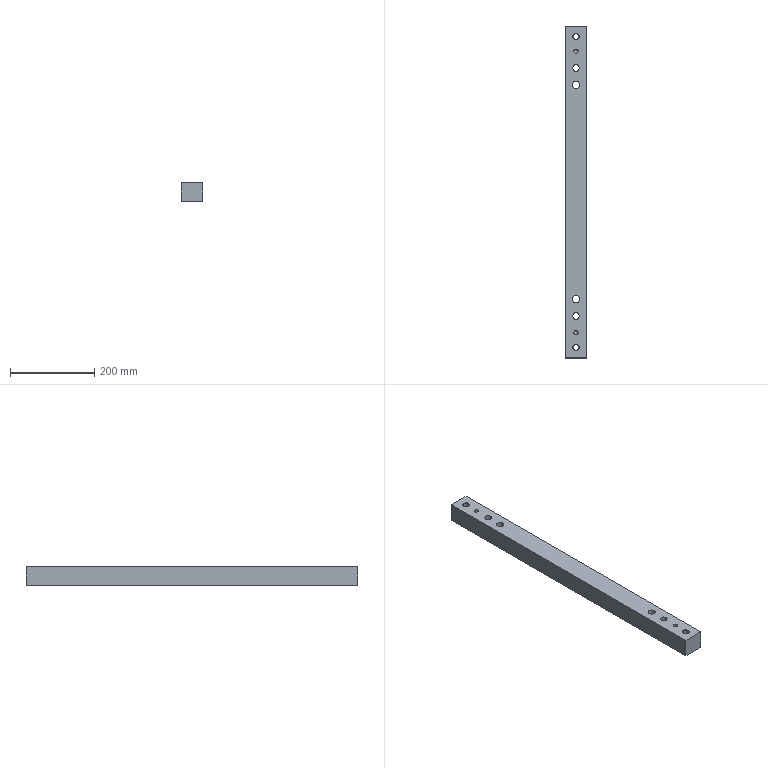Part | STEP file | 026_id2218_x_t | 1 solid | 18 faces | box 50 x 790 x 45 mm | volume 1720407 mm3 | cylinder 8 | plane 6 | cone 4 | commonest cylinder face diameters 10.3 x2 14 x2 16 x2 17 x2
STEP:
#1=CARTESIAN_POINT('',(0.,0.,0.));
#2=DIRECTION('',(0.,0.,1.));
#3=DIRECTION('',(1.,0.,0.));
#4=AXIS2_PLACEMENT_3D('',#1,#2,#3);
#5=CARTESIAN_POINT('',(1285.,-255.,185.));
#6=VERTEX_POINT('',#5);
#7=CARTESIAN_POINT('',(1293.5,-255.,185.));
#8=DIRECTION('',(0.,0.,1.));
#9=DIRECTION('',(-1.,0.,0.));
#10=AXIS2_PLACEMENT_3D('',#7,#8,#9);
#11=CIRCLE('',#10,8.5);
#12=CARTESIAN_POINT('',(193.5,0.,185.));
#13=DIRECTION('',(0.,0.,-1.));
#14=DIRECTION('',(1.,0.,0.));
#15=AXIS2_PLACEMENT_3D('',#12,#13,#14);
#16=PLANE('',#15);
#17=CARTESIAN_POINT('',(1091.5,255.));
#18=CARTESIAN_POINT('',(1091.5,269.722));
#19=CARTESIAN_POINT('',(1104.25,262.361));
#20=CARTESIAN_POINT('',(1117.,255.));
#21=CARTESIAN_POINT('',(1104.25,247.639));
#22=CARTESIAN_POINT('',(1091.5,240.278));
#23=CARTESIAN_POINT('',(1091.5,255.));
#24=(BOUNDED_CURVE()B_SPLINE_CURVE(2,(#17,#18,#19,#20,#21,#22,#23),.UNSPECIFIED.,.T.,.F.)B_SPLINE_CURVE_WITH_KNOTS((1,2,2,2,2,1),(-2.094,0.,2.094,4.189,6.283,8.378),.UNSPECIFIED.)CURVE()GEOMETRIC_REPRESENTATION_ITEM()RATIONAL_B_SPLINE_CURVE((1.,0.5,1.,0.5,1.,0.5,1.))REPRESENTATION_ITEM(''));
#25=(GEOMETRIC_REPRESENTATION_CONTEXT(2)PARAMETRIC_REPRESENTATION_CONTEXT()REPRESENTATION_CONTEXT('',''));
#26=DEFINITIONAL_REPRESENTATION('',(#24),#25);
#27=PCURVE('',#16,#26);
#28=CARTESIAN_POINT('',(1293.5,-255.,150.));
#29=DIRECTION('',(0.,0.,1.));
#30=DIRECTION('',(1.,0.,0.));
#31=AXIS2_PLACEMENT_3D('',#28,#29,#30);
#32=CYLINDRICAL_SURFACE('',#31,8.5);
#33=CARTESIAN_POINT('',(3.142,35.));
#34=DIRECTION('',(1.,0.));
#35=VECTOR('',#34,1.);
#36=LINE('',#33,#35);
#37=(GEOMETRIC_REPRESENTATION_CONTEXT(2)PARAMETRIC_REPRESENTATION_CONTEXT()REPRESENTATION_CONTEXT('',''));
#38=DEFINITIONAL_REPRESENTATION('',(#36),#37);
#39=PCURVE('',#32,#38);
#40=SURFACE_CURVE('',#11,(#27,#39),.PCURVE_S1.);
#41=EDGE_CURVE('',#6,#6,#40,.T.);
#42=ORIENTED_EDGE('',*,*,#41,.T.);
#43=EDGE_LOOP('',(#42));
#44=FACE_BOUND('',#43,.T.);
#45=CARTESIAN_POINT('',(1286.5,-370.,185.));
#46=VERTEX_POINT('',#45);
#47=CARTESIAN_POINT('',(1293.5,-370.,185.));
#48=DIRECTION('',(0.,0.,-1.));
#49=DIRECTION('',(-1.,0.,0.));
#50=AXIS2_PLACEMENT_3D('',#47,#48,#49);
#51=CIRCLE('',#50,7.);
#52=CARTESIAN_POINT('',(1100.,370.));
#53=DIRECTION('',(-1.,0.));
#54=AXIS2_PLACEMENT_2D('',#52,#53);
#55=CIRCLE('',#54,7.);
#56=(GEOMETRIC_REPRESENTATION_CONTEXT(2)PARAMETRIC_REPRESENTATION_CONTEXT()REPRESENTATION_CONTEXT('',''));
#57=DEFINITIONAL_REPRESENTATION('',(#55),#56);
#58=PCURVE('',#16,#57);
#59=CARTESIAN_POINT('',(1293.5,-370.,230.));
#60=DIRECTION('',(0.,0.,-1.));
#61=DIRECTION('',(-1.,0.,0.));
#62=AXIS2_PLACEMENT_3D('',#59,#60,#61);
#63=CYLINDRICAL_SURFACE('',#62,7.);
#64=CARTESIAN_POINT('',(0.,45.));
#65=DIRECTION('',(1.,0.));
#66=VECTOR('',#65,1.);
#67=LINE('',#64,#66);
#68=(GEOMETRIC_REPRESENTATION_CONTEXT(2)PARAMETRIC_REPRESENTATION_CONTEXT()REPRESENTATION_CONTEXT('',''));
#69=DEFINITIONAL_REPRESENTATION('',(#67),#68);
#70=PCURVE('',#63,#69);
#71=SURFACE_CURVE('',#51,(#58,#70),.PCURVE_S1.);
#72=EDGE_CURVE('',#46,#46,#71,.T.);
#73=ORIENTED_EDGE('',*,*,#72,.F.);
#74=EDGE_LOOP('',(#73));
#75=FACE_BOUND('',#74,.T.);
#76=CARTESIAN_POINT('',(1318.5,395.,185.));
#77=VERTEX_POINT('',#76);
#78=CARTESIAN_POINT('',(1318.5,-395.,185.));
#79=VERTEX_POINT('',#78);
#80=CARTESIAN_POINT('',(1318.5,0.,185.));
#81=DIRECTION('',(0.,-1.,0.));
#82=VECTOR('',#81,1.);
#83=LINE('',#80,#82);
#84=CARTESIAN_POINT('',(1125.,0.));
#85=DIRECTION('',(0.,1.));
#86=VECTOR('',#85,1.);
#87=LINE('',#84,#86);
#88=(GEOMETRIC_REPRESENTATION_CONTEXT(2)PARAMETRIC_REPRESENTATION_CONTEXT()REPRESENTATION_CONTEXT('',''));
#89=DEFINITIONAL_REPRESENTATION('',(#87),#88);
#90=PCURVE('',#16,#89);
#91=CARTESIAN_POINT('',(1318.5,-210.,-28.5));
#92=DIRECTION('',(1.,0.,0.));
#93=DIRECTION('',(0.,0.,1.));
#94=AXIS2_PLACEMENT_3D('',#91,#92,#93);
#95=PLANE('',#94);
#96=CARTESIAN_POINT('',(213.5,-210.));
#97=DIRECTION('',(0.,1.));
#98=VECTOR('',#97,1.);
#99=LINE('',#96,#98);
#100=(GEOMETRIC_REPRESENTATION_CONTEXT(2)PARAMETRIC_REPRESENTATION_CONTEXT()REPRESENTATION_CONTEXT('',''));
#101=DEFINITIONAL_REPRESENTATION('',(#99),#100);
#102=PCURVE('',#95,#101);
#103=SURFACE_CURVE('',#83,(#90,#102),.PCURVE_S1.);
#104=EDGE_CURVE('',#77,#79,#103,.T.);
#105=ORIENTED_EDGE('',*,*,#104,.T.);
#106=CARTESIAN_POINT('',(1268.5,-395.,185.));
#107=VERTEX_POINT('',#106);
#108=CARTESIAN_POINT('',(193.5,-395.,185.));
#109=DIRECTION('',(1.,0.,0.));
#110=VECTOR('',#109,1.);
#111=LINE('',#108,#110);
#112=CARTESIAN_POINT('',(0.,395.));
#113=DIRECTION('',(1.,0.));
#114=VECTOR('',#113,1.);
#115=LINE('',#112,#114);
#116=(GEOMETRIC_REPRESENTATION_CONTEXT(2)PARAMETRIC_REPRESENTATION_CONTEXT()REPRESENTATION_CONTEXT('',''));
#117=DEFINITIONAL_REPRESENTATION('',(#115),#116);
#118=PCURVE('',#16,#117);
#119=CARTESIAN_POINT('',(1318.5,-395.,-28.5));
#120=DIRECTION('',(0.,1.,0.));
#121=DIRECTION('',(0.,0.,-1.));
#122=AXIS2_PLACEMENT_3D('',#119,#120,#121);
#123=PLANE('',#122);
#124=CARTESIAN_POINT('',(-213.5,1125.));
#125=DIRECTION('',(0.,-1.));
#126=VECTOR('',#125,1.);
#127=LINE('',#124,#126);
#128=(GEOMETRIC_REPRESENTATION_CONTEXT(2)PARAMETRIC_REPRESENTATION_CONTEXT()REPRESENTATION_CONTEXT('',''));
#129=DEFINITIONAL_REPRESENTATION('',(#127),#128);
#130=PCURVE('',#123,#129);
#131=SURFACE_CURVE('',#111,(#118,#130),.PCURVE_S1.);
#132=EDGE_CURVE('',#107,#79,#131,.T.);
#133=ORIENTED_EDGE('',*,*,#132,.F.);
#134=CARTESIAN_POINT('',(1268.5,395.,185.));
#135=VERTEX_POINT('',#134);
#136=CARTESIAN_POINT('',(1268.5,-210.,185.));
#137=DIRECTION('',(0.,1.,0.));
#138=VECTOR('',#137,1.);
#139=LINE('',#136,#138);
#140=CARTESIAN_POINT('',(1075.,210.));
#141=DIRECTION('',(0.,-1.));
#142=VECTOR('',#141,1.);
#143=LINE('',#140,#142);
#144=(GEOMETRIC_REPRESENTATION_CONTEXT(2)PARAMETRIC_REPRESENTATION_CONTEXT()REPRESENTATION_CONTEXT('',''));
#145=DEFINITIONAL_REPRESENTATION('',(#143),#144);
#146=PCURVE('',#16,#145);
#147=CARTESIAN_POINT('',(1268.5,-210.,-28.5));
#148=DIRECTION('',(1.,0.,0.));
#149=DIRECTION('',(0.,0.,1.));
#150=AXIS2_PLACEMENT_3D('',#147,#148,#149);
#151=PLANE('',#150);
#152=CARTESIAN_POINT('',(213.5,0.));
#153=DIRECTION('',(0.,-1.));
#154=VECTOR('',#153,1.);
#155=LINE('',#152,#154);
#156=(GEOMETRIC_REPRESENTATION_CONTEXT(2)PARAMETRIC_REPRESENTATION_CONTEXT()REPRESENTATION_CONTEXT('',''));
#157=DEFINITIONAL_REPRESENTATION('',(#155),#156);
#158=PCURVE('',#151,#157);
#159=SURFACE_CURVE('',#139,(#146,#158),.PCURVE_S1.);
#160=EDGE_CURVE('',#107,#135,#159,.T.);
#161=ORIENTED_EDGE('',*,*,#160,.T.);
#162=CARTESIAN_POINT('',(193.5,395.,185.));
#163=DIRECTION('',(1.,0.,0.));
#164=VECTOR('',#163,1.);
#165=LINE('',#162,#164);
#166=CARTESIAN_POINT('',(0.,-395.));
#167=DIRECTION('',(1.,0.));
#168=VECTOR('',#167,1.);
#169=LINE('',#166,#168);
#170=(GEOMETRIC_REPRESENTATION_CONTEXT(2)PARAMETRIC_REPRESENTATION_CONTEXT()REPRESENTATION_CONTEXT('',''));
#171=DEFINITIONAL_REPRESENTATION('',(#169),#170);
#172=PCURVE('',#16,#171);
#173=CARTESIAN_POINT('',(1318.5,395.,-28.5));
#174=DIRECTION('',(0.,1.,0.));
#175=DIRECTION('',(0.,0.,-1.));
#176=AXIS2_PLACEMENT_3D('',#173,#174,#175);
#177=PLANE('',#176);
#178=CARTESIAN_POINT('',(-213.5,1125.));
#179=DIRECTION('',(0.,-1.));
#180=VECTOR('',#179,1.);
#181=LINE('',#178,#180);
#182=(GEOMETRIC_REPRESENTATION_CONTEXT(2)PARAMETRIC_REPRESENTATION_CONTEXT()REPRESENTATION_CONTEXT('',''));
#183=DEFINITIONAL_REPRESENTATION('',(#181),#182);
#184=PCURVE('',#177,#183);
#185=SURFACE_CURVE('',#165,(#172,#184),.PCURVE_S1.);
#186=EDGE_CURVE('',#135,#77,#185,.T.);
#187=ORIENTED_EDGE('',*,*,#186,.T.);
#188=EDGE_LOOP('',(#105,#133,#161,#187));
#189=FACE_BOUND('',#188,.T.);
#190=CARTESIAN_POINT('',(1285.5,295.,185.));
#191=VERTEX_POINT('',#190);
#192=CARTESIAN_POINT('',(1293.5,295.,185.));
#193=DIRECTION('',(0.,0.,-1.));
#194=DIRECTION('',(-1.,0.,0.));
#195=AXIS2_PLACEMENT_3D('',#192,#193,#194);
#196=CIRCLE('',#195,8.);
#197=CARTESIAN_POINT('',(1100.,-295.));
#198=DIRECTION('',(-1.,0.));
#199=AXIS2_PLACEMENT_2D('',#197,#198);
#200=CIRCLE('',#199,8.);
#201=(GEOMETRIC_REPRESENTATION_CONTEXT(2)PARAMETRIC_REPRESENTATION_CONTEXT()REPRESENTATION_CONTEXT('',''));
#202=DEFINITIONAL_REPRESENTATION('',(#200),#201);
#203=PCURVE('',#16,#202);
#204=CARTESIAN_POINT('',(1293.5,295.,310.));
#205=DIRECTION('',(0.,0.,-1.));
#206=DIRECTION('',(-1.,0.,0.));
#207=AXIS2_PLACEMENT_3D('',#204,#205,#206);
#208=CYLINDRICAL_SURFACE('',#207,8.);
#209=CARTESIAN_POINT('',(0.,125.));
#210=DIRECTION('',(1.,0.));
#211=VECTOR('',#210,1.);
#212=LINE('',#209,#211);
#213=(GEOMETRIC_REPRESENTATION_CONTEXT(2)PARAMETRIC_REPRESENTATION_CONTEXT()REPRESENTATION_CONTEXT('',''));
#214=DEFINITIONAL_REPRESENTATION('',(#212),#213);
#215=PCURVE('',#208,#214);
#216=SURFACE_CURVE('',#196,(#203,#215),.PCURVE_S1.);
#217=EDGE_CURVE('',#191,#191,#216,.T.);
#218=ORIENTED_EDGE('',*,*,#217,.F.);
#219=EDGE_LOOP('',(#218));
#220=FACE_BOUND('',#219,.T.);
#221=CARTESIAN_POINT('',(1285.5,-295.,185.));
#222=VERTEX_POINT('',#221);
#223=CARTESIAN_POINT('',(1293.5,-295.,185.));
#224=DIRECTION('',(0.,0.,-1.));
#225=DIRECTION('',(-1.,0.,0.));
#226=AXIS2_PLACEMENT_3D('',#223,#224,#225);
#227=CIRCLE('',#226,8.);
#228=CARTESIAN_POINT('',(1100.,295.));
#229=DIRECTION('',(-1.,0.));
#230=AXIS2_PLACEMENT_2D('',#228,#229);
#231=CIRCLE('',#230,8.);
#232=(GEOMETRIC_REPRESENTATION_CONTEXT(2)PARAMETRIC_REPRESENTATION_CONTEXT()REPRESENTATION_CONTEXT('',''));
#233=DEFINITIONAL_REPRESENTATION('',(#231),#232);
#234=PCURVE('',#16,#233);
#235=CARTESIAN_POINT('',(1293.5,-295.,310.));
#236=DIRECTION('',(0.,0.,-1.));
#237=DIRECTION('',(-1.,0.,0.));
#238=AXIS2_PLACEMENT_3D('',#235,#236,#237);
#239=CYLINDRICAL_SURFACE('',#238,8.);
#240=CARTESIAN_POINT('',(0.,125.));
#241=DIRECTION('',(1.,0.));
#242=VECTOR('',#241,1.);
#243=LINE('',#240,#242);
#244=(GEOMETRIC_REPRESENTATION_CONTEXT(2)PARAMETRIC_REPRESENTATION_CONTEXT()REPRESENTATION_CONTEXT('',''));
#245=DEFINITIONAL_REPRESENTATION('',(#243),#244);
#246=PCURVE('',#239,#245);
#247=SURFACE_CURVE('',#227,(#234,#246),.PCURVE_S1.);
#248=EDGE_CURVE('',#222,#222,#247,.T.);
#249=ORIENTED_EDGE('',*,*,#248,.F.);
#250=EDGE_LOOP('',(#249));
#251=FACE_BOUND('',#250,.T.);
#252=CARTESIAN_POINT('',(1286.5,370.,185.));
#253=VERTEX_POINT('',#252);
#254=CARTESIAN_POINT('',(1293.5,370.,185.));
#255=DIRECTION('',(0.,0.,-1.));
#256=DIRECTION('',(-1.,0.,0.));
#257=AXIS2_PLACEMENT_3D('',#254,#255,#256);
#258=CIRCLE('',#257,7.);
#259=CARTESIAN_POINT('',(1100.,-370.));
#260=DIRECTION('',(-1.,0.));
#261=AXIS2_PLACEMENT_2D('',#259,#260);
#262=CIRCLE('',#261,7.);
#263=(GEOMETRIC_REPRESENTATION_CONTEXT(2)PARAMETRIC_REPRESENTATION_CONTEXT()REPRESENTATION_CONTEXT('',''));
#264=DEFINITIONAL_REPRESENTATION('',(#262),#263);
#265=PCURVE('',#16,#264);
#266=CARTESIAN_POINT('',(1293.5,370.,230.));
#267=DIRECTION('',(0.,0.,-1.));
#268=DIRECTION('',(-1.,0.,0.));
#269=AXIS2_PLACEMENT_3D('',#266,#267,#268);
#270=CYLINDRICAL_SURFACE('',#269,7.);
#271=CARTESIAN_POINT('',(0.,45.));
#272=DIRECTION('',(1.,0.));
#273=VECTOR('',#272,1.);
#274=LINE('',#271,#273);
#275=(GEOMETRIC_REPRESENTATION_CONTEXT(2)PARAMETRIC_REPRESENTATION_CONTEXT()REPRESENTATION_CONTEXT('',''));
#276=DEFINITIONAL_REPRESENTATION('',(#274),#275);
#277=PCURVE('',#270,#276);
#278=SURFACE_CURVE('',#258,(#265,#277),.PCURVE_S1.);
#279=EDGE_CURVE('',#253,#253,#278,.T.);
#280=ORIENTED_EDGE('',*,*,#279,.F.);
#281=EDGE_LOOP('',(#280));
#282=FACE_BOUND('',#281,.T.);
#283=CARTESIAN_POINT('',(1285.,255.,185.));
#284=VERTEX_POINT('',#283);
#285=CARTESIAN_POINT('',(1293.5,255.,185.));
#286=DIRECTION('',(0.,0.,1.));
#287=DIRECTION('',(-1.,0.,0.));
#288=AXIS2_PLACEMENT_3D('',#285,#286,#287);
#289=CIRCLE('',#288,8.5);
#290=CARTESIAN_POINT('',(1091.5,-255.));
#291=CARTESIAN_POINT('',(1091.5,-240.278));
#292=CARTESIAN_POINT('',(1104.25,-247.639));
#293=CARTESIAN_POINT('',(1117.,-255.));
#294=CARTESIAN_POINT('',(1104.25,-262.361));
#295=CARTESIAN_POINT('',(1091.5,-269.722));
#296=CARTESIAN_POINT('',(1091.5,-255.));
#297=(BOUNDED_CURVE()B_SPLINE_CURVE(2,(#290,#291,#292,#293,#294,#295,#296),.UNSPECIFIED.,.T.,.F.)B_SPLINE_CURVE_WITH_KNOTS((1,2,2,2,2,1),(-2.094,0.,2.094,4.189,6.283,8.378),.UNSPECIFIED.)CURVE()GEOMETRIC_REPRESENTATION_ITEM()RATIONAL_B_SPLINE_CURVE((1.,0.5,1.,0.5,1.,0.5,1.))REPRESENTATION_ITEM(''));
#298=(GEOMETRIC_REPRESENTATION_CONTEXT(2)PARAMETRIC_REPRESENTATION_CONTEXT()REPRESENTATION_CONTEXT('',''));
#299=DEFINITIONAL_REPRESENTATION('',(#297),#298);
#300=PCURVE('',#16,#299);
#301=CARTESIAN_POINT('',(1293.5,255.,150.));
#302=DIRECTION('',(0.,0.,1.));
#303=DIRECTION('',(1.,0.,0.));
#304=AXIS2_PLACEMENT_3D('',#301,#302,#303);
#305=CYLINDRICAL_SURFACE('',#304,8.5);
#306=CARTESIAN_POINT('',(3.142,35.));
#307=DIRECTION('',(1.,0.));
#308=VECTOR('',#307,1.);
#309=LINE('',#306,#308);
#310=(GEOMETRIC_REPRESENTATION_CONTEXT(2)PARAMETRIC_REPRESENTATION_CONTEXT()REPRESENTATION_CONTEXT('',''));
#311=DEFINITIONAL_REPRESENTATION('',(#309),#310);
#312=PCURVE('',#305,#311);
#313=SURFACE_CURVE('',#289,(#300,#312),.PCURVE_S1.);
#314=EDGE_CURVE('',#284,#284,#313,.T.);
#315=ORIENTED_EDGE('',*,*,#314,.T.);
#316=EDGE_LOOP('',(#315));
#317=FACE_BOUND('',#316,.T.);
#318=ADVANCED_FACE('',(#44,#75,#189,#220,#251,#282,#317),#16,.T.);
#319=CARTESIAN_POINT('',(1288.35,-335.,230.));
#320=VERTEX_POINT('',#319);
#321=CARTESIAN_POINT('',(1293.5,-335.,230.));
#322=DIRECTION('',(0.,0.,-1.));
#323=DIRECTION('',(-1.,0.,0.));
#324=AXIS2_PLACEMENT_3D('',#321,#322,#323);
#325=CIRCLE('',#324,5.15);
#326=CARTESIAN_POINT('',(1318.5,-210.,230.));
#327=DIRECTION('',(0.,0.,-1.));
#328=DIRECTION('',(0.,-1.,0.));
#329=AXIS2_PLACEMENT_3D('',#326,#327,#328);
#330=PLANE('',#329);
#331=CARTESIAN_POINT('',(125.,25.));
#332=DIRECTION('',(0.,1.));
#333=AXIS2_PLACEMENT_2D('',#331,#332);
#334=CIRCLE('',#333,5.15);
#335=(GEOMETRIC_REPRESENTATION_CONTEXT(2)PARAMETRIC_REPRESENTATION_CONTEXT()REPRESENTATION_CONTEXT('',''));
#336=DEFINITIONAL_REPRESENTATION('',(#334),#335);
#337=PCURVE('',#330,#336);
#338=CARTESIAN_POINT('',(1293.5,-335.,259.));
#339=DIRECTION('',(0.,0.,-1.));
#340=DIRECTION('',(-1.,0.,0.));
#341=AXIS2_PLACEMENT_3D('',#338,#339,#340);
#342=CYLINDRICAL_SURFACE('',#341,5.15);
#343=CARTESIAN_POINT('',(0.,29.));
#344=DIRECTION('',(1.,0.));
#345=VECTOR('',#344,1.);
#346=LINE('',#343,#345);
#347=(GEOMETRIC_REPRESENTATION_CONTEXT(2)PARAMETRIC_REPRESENTATION_CONTEXT()REPRESENTATION_CONTEXT('',''));
#348=DEFINITIONAL_REPRESENTATION('',(#346),#347);
#349=PCURVE('',#342,#348);
#350=SURFACE_CURVE('',#325,(#337,#349),.PCURVE_S1.);
#351=EDGE_CURVE('',#320,#320,#350,.T.);
#352=ORIENTED_EDGE('',*,*,#351,.T.);
#353=EDGE_LOOP('',(#352));
#354=FACE_BOUND('',#353,.T.);
#355=CARTESIAN_POINT('',(1288.35,335.,230.));
#356=VERTEX_POINT('',#355);
#357=CARTESIAN_POINT('',(1293.5,335.,230.));
#358=DIRECTION('',(0.,0.,1.));
#359=DIRECTION('',(-1.,0.,0.));
#360=AXIS2_PLACEMENT_3D('',#357,#358,#359);
#361=CIRCLE('',#360,5.15);
#362=CARTESIAN_POINT('',(-545.,30.15));
#363=CARTESIAN_POINT('',(-536.08,30.15));
#364=CARTESIAN_POINT('',(-540.54,22.425));
#365=CARTESIAN_POINT('',(-545.,14.7));
#366=CARTESIAN_POINT('',(-549.46,22.425));
#367=CARTESIAN_POINT('',(-553.92,30.15));
#368=CARTESIAN_POINT('',(-545.,30.15));
#369=(BOUNDED_CURVE()B_SPLINE_CURVE(2,(#362,#363,#364,#365,#366,#367,#368),.UNSPECIFIED.,.T.,.F.)B_SPLINE_CURVE_WITH_KNOTS((1,2,2,2,2,1),(-2.094,0.,2.094,4.189,6.283,8.378),.UNSPECIFIED.)CURVE()GEOMETRIC_REPRESENTATION_ITEM()RATIONAL_B_SPLINE_CURVE((1.,0.5,1.,0.5,1.,0.5,1.))REPRESENTATION_ITEM(''));
#370=(GEOMETRIC_REPRESENTATION_CONTEXT(2)PARAMETRIC_REPRESENTATION_CONTEXT()REPRESENTATION_CONTEXT('',''));
#371=DEFINITIONAL_REPRESENTATION('',(#369),#370);
#372=PCURVE('',#330,#371);
#373=CARTESIAN_POINT('',(1293.5,335.,259.));
#374=DIRECTION('',(0.,0.,-1.));
#375=DIRECTION('',(-1.,0.,0.));
#376=AXIS2_PLACEMENT_3D('',#373,#374,#375);
#377=CYLINDRICAL_SURFACE('',#376,5.15);
#378=CARTESIAN_POINT('',(6.283,29.));
#379=DIRECTION('',(-1.,0.));
#380=VECTOR('',#379,1.);
#381=LINE('',#378,#380);
#382=(GEOMETRIC_REPRESENTATION_CONTEXT(2)PARAMETRIC_REPRESENTATION_CONTEXT()REPRESENTATION_CONTEXT('',''));
#383=DEFINITIONAL_REPRESENTATION('',(#381),#382);
#384=PCURVE('',#377,#383);
#385=SURFACE_CURVE('',#361,(#372,#384),.PCURVE_S1.);
#386=EDGE_CURVE('',#356,#356,#385,.T.);
#387=ORIENTED_EDGE('',*,*,#386,.F.);
#388=EDGE_LOOP('',(#387));
#389=FACE_BOUND('',#388,.T.);
#390=CARTESIAN_POINT('',(1285.,255.,230.));
#391=VERTEX_POINT('',#390);
#392=CARTESIAN_POINT('',(1293.5,255.,230.));
#393=DIRECTION('',(0.,0.,1.));
#394=DIRECTION('',(-1.,0.,0.));
#395=AXIS2_PLACEMENT_3D('',#392,#393,#394);
#396=CIRCLE('',#395,8.5);
#397=CARTESIAN_POINT('',(-465.,33.5));
#398=CARTESIAN_POINT('',(-450.278,33.5));
#399=CARTESIAN_POINT('',(-457.639,20.75));
#400=CARTESIAN_POINT('',(-465.,8.));
#401=CARTESIAN_POINT('',(-472.361,20.75));
#402=CARTESIAN_POINT('',(-479.722,33.5));
#403=CARTESIAN_POINT('',(-465.,33.5));
#404=(BOUNDED_CURVE()B_SPLINE_CURVE(2,(#397,#398,#399,#400,#401,#402,#403),.UNSPECIFIED.,.T.,.F.)B_SPLINE_CURVE_WITH_KNOTS((1,2,2,2,2,1),(-2.094,0.,2.094,4.189,6.283,8.378),.UNSPECIFIED.)CURVE()GEOMETRIC_REPRESENTATION_ITEM()RATIONAL_B_SPLINE_CURVE((1.,0.5,1.,0.5,1.,0.5,1.))REPRESENTATION_ITEM(''));
#405=(GEOMETRIC_REPRESENTATION_CONTEXT(2)PARAMETRIC_REPRESENTATION_CONTEXT()REPRESENTATION_CONTEXT('',''));
#406=DEFINITIONAL_REPRESENTATION('',(#404),#405);
#407=PCURVE('',#330,#406);
#408=CARTESIAN_POINT('',(3.142,80.));
#409=DIRECTION('',(1.,0.));
#410=VECTOR('',#409,1.);
#411=LINE('',#408,#410);
#412=(GEOMETRIC_REPRESENTATION_CONTEXT(2)PARAMETRIC_REPRESENTATION_CONTEXT()REPRESENTATION_CONTEXT('',''));
#413=DEFINITIONAL_REPRESENTATION('',(#411),#412);
#414=PCURVE('',#305,#413);
#415=SURFACE_CURVE('',#396,(#407,#414),.PCURVE_S1.);
#416=EDGE_CURVE('',#391,#391,#415,.T.);
#417=ORIENTED_EDGE('',*,*,#416,.F.);
#418=EDGE_LOOP('',(#417));
#419=FACE_BOUND('',#418,.T.);
#420=CARTESIAN_POINT('',(1318.5,-395.,230.));
#421=VERTEX_POINT('',#420);
#422=CARTESIAN_POINT('',(1268.5,-395.,230.));
#423=VERTEX_POINT('',#422);
#424=CARTESIAN_POINT('',(1318.5,-395.,230.));
#425=DIRECTION('',(-1.,0.,0.));
#426=VECTOR('',#425,1.);
#427=LINE('',#424,#426);
#428=CARTESIAN_POINT('',(185.,0.));
#429=DIRECTION('',(0.,1.));
#430=VECTOR('',#429,1.);
#431=LINE('',#428,#430);
#432=(GEOMETRIC_REPRESENTATION_CONTEXT(2)PARAMETRIC_REPRESENTATION_CONTEXT()REPRESENTATION_CONTEXT('',''));
#433=DEFINITIONAL_REPRESENTATION('',(#431),#432);
#434=PCURVE('',#330,#433);
#435=CARTESIAN_POINT('',(-258.5,0.));
#436=DIRECTION('',(0.,1.));
#437=VECTOR('',#436,1.);
#438=LINE('',#435,#437);
#439=(GEOMETRIC_REPRESENTATION_CONTEXT(2)PARAMETRIC_REPRESENTATION_CONTEXT()REPRESENTATION_CONTEXT('',''));
#440=DEFINITIONAL_REPRESENTATION('',(#438),#439);
#441=PCURVE('',#123,#440);
#442=SURFACE_CURVE('',#427,(#434,#441),.PCURVE_S1.);
#443=EDGE_CURVE('',#421,#423,#442,.T.);
#444=ORIENTED_EDGE('',*,*,#443,.F.);
#445=CARTESIAN_POINT('',(1318.5,395.,230.));
#446=VERTEX_POINT('',#445);
#447=CARTESIAN_POINT('',(1318.5,-210.,230.));
#448=DIRECTION('',(0.,-1.,0.));
#449=VECTOR('',#448,1.);
#450=LINE('',#447,#449);
#451=CARTESIAN_POINT('',(0.,0.));
#452=DIRECTION('',(1.,0.));
#453=VECTOR('',#452,1.);
#454=LINE('',#451,#453);
#455=(GEOMETRIC_REPRESENTATION_CONTEXT(2)PARAMETRIC_REPRESENTATION_CONTEXT()REPRESENTATION_CONTEXT('',''));
#456=DEFINITIONAL_REPRESENTATION('',(#454),#455);
#457=PCURVE('',#330,#456);
#458=CARTESIAN_POINT('',(258.5,0.));
#459=DIRECTION('',(0.,1.));
#460=VECTOR('',#459,1.);
#461=LINE('',#458,#460);
#462=(GEOMETRIC_REPRESENTATION_CONTEXT(2)PARAMETRIC_REPRESENTATION_CONTEXT()REPRESENTATION_CONTEXT('',''));
#463=DEFINITIONAL_REPRESENTATION('',(#461),#462);
#464=PCURVE('',#95,#463);
#465=SURFACE_CURVE('',#450,(#457,#464),.PCURVE_S1.);
#466=EDGE_CURVE('',#446,#421,#465,.T.);
#467=ORIENTED_EDGE('',*,*,#466,.F.);
#468=CARTESIAN_POINT('',(1268.5,395.,230.));
#469=VERTEX_POINT('',#468);
#470=CARTESIAN_POINT('',(1318.5,395.,230.));
#471=DIRECTION('',(-1.,0.,0.));
#472=VECTOR('',#471,1.);
#473=LINE('',#470,#472);
#474=CARTESIAN_POINT('',(-605.,0.));
#475=DIRECTION('',(0.,1.));
#476=VECTOR('',#475,1.);
#477=LINE('',#474,#476);
#478=(GEOMETRIC_REPRESENTATION_CONTEXT(2)PARAMETRIC_REPRESENTATION_CONTEXT()REPRESENTATION_CONTEXT('',''));
#479=DEFINITIONAL_REPRESENTATION('',(#477),#478);
#480=PCURVE('',#330,#479);
#481=CARTESIAN_POINT('',(-258.5,0.));
#482=DIRECTION('',(0.,1.));
#483=VECTOR('',#482,1.);
#484=LINE('',#481,#483);
#485=(GEOMETRIC_REPRESENTATION_CONTEXT(2)PARAMETRIC_REPRESENTATION_CONTEXT()REPRESENTATION_CONTEXT('',''));
#486=DEFINITIONAL_REPRESENTATION('',(#484),#485);
#487=PCURVE('',#177,#486);
#488=SURFACE_CURVE('',#473,(#480,#487),.PCURVE_S1.);
#489=EDGE_CURVE('',#446,#469,#488,.T.);
#490=ORIENTED_EDGE('',*,*,#489,.T.);
#491=CARTESIAN_POINT('',(1268.5,-210.,230.));
#492=DIRECTION('',(0.,-1.,0.));
#493=VECTOR('',#492,1.);
#494=LINE('',#491,#493);
#495=CARTESIAN_POINT('',(0.,50.));
#496=DIRECTION('',(1.,0.));
#497=VECTOR('',#496,1.);
#498=LINE('',#495,#497);
#499=(GEOMETRIC_REPRESENTATION_CONTEXT(2)PARAMETRIC_REPRESENTATION_CONTEXT()REPRESENTATION_CONTEXT('',''));
#500=DEFINITIONAL_REPRESENTATION('',(#498),#499);
#501=PCURVE('',#330,#500);
#502=CARTESIAN_POINT('',(258.5,0.));
#503=DIRECTION('',(0.,1.));
#504=VECTOR('',#503,1.);
#505=LINE('',#502,#504);
#506=(GEOMETRIC_REPRESENTATION_CONTEXT(2)PARAMETRIC_REPRESENTATION_CONTEXT()REPRESENTATION_CONTEXT('',''));
#507=DEFINITIONAL_REPRESENTATION('',(#505),#506);
#508=PCURVE('',#151,#507);
#509=SURFACE_CURVE('',#494,(#501,#508),.PCURVE_S1.);
#510=EDGE_CURVE('',#469,#423,#509,.T.);
#511=ORIENTED_EDGE('',*,*,#510,.T.);
#512=EDGE_LOOP('',(#444,#467,#490,#511));
#513=FACE_BOUND('',#512,.T.);
#514=CARTESIAN_POINT('',(1285.5,-295.,230.));
#515=VERTEX_POINT('',#514);
#516=CARTESIAN_POINT('',(1293.5,-295.,230.));
#517=DIRECTION('',(0.,0.,-1.));
#518=DIRECTION('',(-1.,0.,0.));
#519=AXIS2_PLACEMENT_3D('',#516,#517,#518);
#520=CIRCLE('',#519,8.);
#521=CARTESIAN_POINT('',(85.,25.));
#522=DIRECTION('',(0.,1.));
#523=AXIS2_PLACEMENT_2D('',#521,#522);
#524=CIRCLE('',#523,8.);
#525=(GEOMETRIC_REPRESENTATION_CONTEXT(2)PARAMETRIC_REPRESENTATION_CONTEXT()REPRESENTATION_CONTEXT('',''));
#526=DEFINITIONAL_REPRESENTATION('',(#524),#525);
#527=PCURVE('',#330,#526);
#528=CARTESIAN_POINT('',(0.,80.));
#529=DIRECTION('',(1.,0.));
#530=VECTOR('',#529,1.);
#531=LINE('',#528,#530);
#532=(GEOMETRIC_REPRESENTATION_CONTEXT(2)PARAMETRIC_REPRESENTATION_CONTEXT()REPRESENTATION_CONTEXT('',''));
#533=DEFINITIONAL_REPRESENTATION('',(#531),#532);
#534=PCURVE('',#239,#533);
#535=SURFACE_CURVE('',#520,(#527,#534),.PCURVE_S1.);
#536=EDGE_CURVE('',#515,#515,#535,.T.);
#537=ORIENTED_EDGE('',*,*,#536,.T.);
#538=EDGE_LOOP('',(#537));
#539=FACE_BOUND('',#538,.T.);
#540=CARTESIAN_POINT('',(1285.5,-370.,230.));
#541=VERTEX_POINT('',#540);
#542=CARTESIAN_POINT('',(1293.5,-370.,230.));
#543=DIRECTION('',(0.,0.,-1.));
#544=DIRECTION('',(-1.,0.,0.));
#545=AXIS2_PLACEMENT_3D('',#542,#543,#544);
#546=CIRCLE('',#545,8.);
#547=CARTESIAN_POINT('',(160.,25.));
#548=DIRECTION('',(0.,1.));
#549=AXIS2_PLACEMENT_2D('',#547,#548);
#550=CIRCLE('',#549,8.);
#551=(GEOMETRIC_REPRESENTATION_CONTEXT(2)PARAMETRIC_REPRESENTATION_CONTEXT()REPRESENTATION_CONTEXT('',''));
#552=DEFINITIONAL_REPRESENTATION('',(#550),#551);
#553=PCURVE('',#330,#552);
#554=CARTESIAN_POINT('',(1293.5,-370.,230.));
#555=DIRECTION('',(0.,0.,1.));
#556=DIRECTION('',(1.,0.,0.));
#557=AXIS2_PLACEMENT_3D('',#554,#555,#556);
#558=CONICAL_SURFACE('',#557,8.,0.7854);
#559=CARTESIAN_POINT('',(9.425,0.));
#560=DIRECTION('',(-1.,0.));
#561=VECTOR('',#560,1.);
#562=LINE('',#559,#561);
#563=(GEOMETRIC_REPRESENTATION_CONTEXT(2)PARAMETRIC_REPRESENTATION_CONTEXT()REPRESENTATION_CONTEXT('',''));
#564=DEFINITIONAL_REPRESENTATION('',(#562),#563);
#565=PCURVE('',#558,#564);
#566=SURFACE_CURVE('',#546,(#553,#565),.PCURVE_S1.);
#567=EDGE_CURVE('',#541,#541,#566,.T.);
#568=ORIENTED_EDGE('',*,*,#567,.T.);
#569=EDGE_LOOP('',(#568));
#570=FACE_BOUND('',#569,.T.);
#571=CARTESIAN_POINT('',(1285.5,370.,230.));
#572=VERTEX_POINT('',#571);
#573=CARTESIAN_POINT('',(1293.5,370.,230.));
#574=DIRECTION('',(0.,0.,-1.));
#575=DIRECTION('',(-1.,0.,0.));
#576=AXIS2_PLACEMENT_3D('',#573,#574,#575);
#577=CIRCLE('',#576,8.);
#578=CARTESIAN_POINT('',(-580.,25.));
#579=DIRECTION('',(0.,1.));
#580=AXIS2_PLACEMENT_2D('',#578,#579);
#581=CIRCLE('',#580,8.);
#582=(GEOMETRIC_REPRESENTATION_CONTEXT(2)PARAMETRIC_REPRESENTATION_CONTEXT()REPRESENTATION_CONTEXT('',''));
#583=DEFINITIONAL_REPRESENTATION('',(#581),#582);
#584=PCURVE('',#330,#583);
#585=CARTESIAN_POINT('',(1293.5,370.,230.));
#586=DIRECTION('',(0.,0.,1.));
#587=DIRECTION('',(1.,0.,0.));
#588=AXIS2_PLACEMENT_3D('',#585,#586,#587);
#589=CONICAL_SURFACE('',#588,8.,0.7854);
#590=CARTESIAN_POINT('',(9.425,0.));
#591=DIRECTION('',(-1.,0.));
#592=VECTOR('',#591,1.);
#593=LINE('',#590,#592);
#594=(GEOMETRIC_REPRESENTATION_CONTEXT(2)PARAMETRIC_REPRESENTATION_CONTEXT()REPRESENTATION_CONTEXT('',''));
#595=DEFINITIONAL_REPRESENTATION('',(#593),#594);
#596=PCURVE('',#589,#595);
#597=SURFACE_CURVE('',#577,(#584,#596),.PCURVE_S1.);
#598=EDGE_CURVE('',#572,#572,#597,.T.);
#599=ORIENTED_EDGE('',*,*,#598,.T.);
#600=EDGE_LOOP('',(#599));
#601=FACE_BOUND('',#600,.T.);
#602=CARTESIAN_POINT('',(1285.5,295.,230.));
#603=VERTEX_POINT('',#602);
#604=CARTESIAN_POINT('',(1293.5,295.,230.));
#605=DIRECTION('',(0.,0.,1.));
#606=DIRECTION('',(1.,0.,0.));
#607=AXIS2_PLACEMENT_3D('',#604,#605,#606);
#608=CIRCLE('',#607,8.);
#609=CARTESIAN_POINT('',(-505.,17.));
#610=CARTESIAN_POINT('',(-518.856,17.));
#611=CARTESIAN_POINT('',(-511.928,29.));
#612=CARTESIAN_POINT('',(-505.,41.));
#613=CARTESIAN_POINT('',(-498.072,29.));
#614=CARTESIAN_POINT('',(-491.144,17.));
#615=CARTESIAN_POINT('',(-505.,17.));
#616=(BOUNDED_CURVE()B_SPLINE_CURVE(2,(#609,#610,#611,#612,#613,#614,#615),.UNSPECIFIED.,.T.,.F.)B_SPLINE_CURVE_WITH_KNOTS((1,2,2,2,2,1),(-2.094,0.,2.094,4.189,6.283,8.378),.UNSPECIFIED.)CURVE()GEOMETRIC_REPRESENTATION_ITEM()RATIONAL_B_SPLINE_CURVE((1.,0.5,1.,0.5,1.,0.5,1.))REPRESENTATION_ITEM(''));
#617=(GEOMETRIC_REPRESENTATION_CONTEXT(2)PARAMETRIC_REPRESENTATION_CONTEXT()REPRESENTATION_CONTEXT('',''));
#618=DEFINITIONAL_REPRESENTATION('',(#616),#617);
#619=PCURVE('',#330,#618);
#620=CARTESIAN_POINT('',(9.425,80.));
#621=DIRECTION('',(-1.,0.));
#622=VECTOR('',#621,1.);
#623=LINE('',#620,#622);
#624=(GEOMETRIC_REPRESENTATION_CONTEXT(2)PARAMETRIC_REPRESENTATION_CONTEXT()REPRESENTATION_CONTEXT('',''));
#625=DEFINITIONAL_REPRESENTATION('',(#623),#624);
#626=PCURVE('',#208,#625);
#627=SURFACE_CURVE('',#608,(#619,#626),.PCURVE_S1.);
#628=EDGE_CURVE('',#603,#603,#627,.T.);
#629=ORIENTED_EDGE('',*,*,#628,.F.);
#630=EDGE_LOOP('',(#629));
#631=FACE_BOUND('',#630,.T.);
#632=CARTESIAN_POINT('',(1285.,-255.,230.));
#633=VERTEX_POINT('',#632);
#634=CARTESIAN_POINT('',(1293.5,-255.,230.));
#635=DIRECTION('',(0.,0.,1.));
#636=DIRECTION('',(-1.,0.,0.));
#637=AXIS2_PLACEMENT_3D('',#634,#635,#636);
#638=CIRCLE('',#637,8.5);
#639=CARTESIAN_POINT('',(45.,33.5));
#640=CARTESIAN_POINT('',(59.722,33.5));
#641=CARTESIAN_POINT('',(52.361,20.75));
#642=CARTESIAN_POINT('',(45.,8.));
#643=CARTESIAN_POINT('',(37.639,20.75));
#644=CARTESIAN_POINT('',(30.278,33.5));
#645=CARTESIAN_POINT('',(45.,33.5));
#646=(BOUNDED_CURVE()B_SPLINE_CURVE(2,(#639,#640,#641,#642,#643,#644,#645),.UNSPECIFIED.,.T.,.F.)B_SPLINE_CURVE_WITH_KNOTS((1,2,2,2,2,1),(-2.094,0.,2.094,4.189,6.283,8.378),.UNSPECIFIED.)CURVE()GEOMETRIC_REPRESENTATION_ITEM()RATIONAL_B_SPLINE_CURVE((1.,0.5,1.,0.5,1.,0.5,1.))REPRESENTATION_ITEM(''));
#647=(GEOMETRIC_REPRESENTATION_CONTEXT(2)PARAMETRIC_REPRESENTATION_CONTEXT()REPRESENTATION_CONTEXT('',''));
#648=DEFINITIONAL_REPRESENTATION('',(#646),#647);
#649=PCURVE('',#330,#648);
#650=CARTESIAN_POINT('',(3.142,80.));
#651=DIRECTION('',(1.,0.));
#652=VECTOR('',#651,1.);
#653=LINE('',#650,#652);
#654=(GEOMETRIC_REPRESENTATION_CONTEXT(2)PARAMETRIC_REPRESENTATION_CONTEXT()REPRESENTATION_CONTEXT('',''));
#655=DEFINITIONAL_REPRESENTATION('',(#653),#654);
#656=PCURVE('',#32,#655);
#657=SURFACE_CURVE('',#638,(#649,#656),.PCURVE_S1.);
#658=EDGE_CURVE('',#633,#633,#657,.T.);
#659=ORIENTED_EDGE('',*,*,#658,.F.);
#660=EDGE_LOOP('',(#659));
#661=FACE_BOUND('',#660,.T.);
#662=ADVANCED_FACE('',(#354,#389,#419,#513,#539,#570,#601,#631,#661),#330,.F.);
#663=ORIENTED_EDGE('',*,*,#132,.T.);
#664=CARTESIAN_POINT('',(1318.5,-395.,-28.5));
#665=DIRECTION('',(0.,0.,-1.));
#666=VECTOR('',#665,1.);
#667=LINE('',#664,#666);
#668=CARTESIAN_POINT('',(0.,0.));
#669=DIRECTION('',(1.,0.));
#670=VECTOR('',#669,1.);
#671=LINE('',#668,#670);
#672=(GEOMETRIC_REPRESENTATION_CONTEXT(2)PARAMETRIC_REPRESENTATION_CONTEXT()REPRESENTATION_CONTEXT('',''));
#673=DEFINITIONAL_REPRESENTATION('',(#671),#672);
#674=PCURVE('',#123,#673);
#675=CARTESIAN_POINT('',(0.,185.));
#676=DIRECTION('',(-1.,0.));
#677=VECTOR('',#676,1.);
#678=LINE('',#675,#677);
#679=(GEOMETRIC_REPRESENTATION_CONTEXT(2)PARAMETRIC_REPRESENTATION_CONTEXT()REPRESENTATION_CONTEXT('',''));
#680=DEFINITIONAL_REPRESENTATION('',(#678),#679);
#681=PCURVE('',#95,#680);
#682=SURFACE_CURVE('',#667,(#674,#681),.PCURVE_S1.);
#683=EDGE_CURVE('',#421,#79,#682,.T.);
#684=ORIENTED_EDGE('',*,*,#683,.F.);
#685=ORIENTED_EDGE('',*,*,#443,.T.);
#686=CARTESIAN_POINT('',(1268.5,-395.,-28.5));
#687=DIRECTION('',(0.,0.,-1.));
#688=VECTOR('',#687,1.);
#689=LINE('',#686,#688);
#690=CARTESIAN_POINT('',(0.,50.));
#691=DIRECTION('',(1.,0.));
#692=VECTOR('',#691,1.);
#693=LINE('',#690,#692);
#694=(GEOMETRIC_REPRESENTATION_CONTEXT(2)PARAMETRIC_REPRESENTATION_CONTEXT()REPRESENTATION_CONTEXT('',''));
#695=DEFINITIONAL_REPRESENTATION('',(#693),#694);
#696=PCURVE('',#123,#695);
#697=CARTESIAN_POINT('',(0.,185.));
#698=DIRECTION('',(-1.,0.));
#699=VECTOR('',#698,1.);
#700=LINE('',#697,#699);
#701=(GEOMETRIC_REPRESENTATION_CONTEXT(2)PARAMETRIC_REPRESENTATION_CONTEXT()REPRESENTATION_CONTEXT('',''));
#702=DEFINITIONAL_REPRESENTATION('',(#700),#701);
#703=PCURVE('',#151,#702);
#704=SURFACE_CURVE('',#689,(#696,#703),.PCURVE_S1.);
#705=EDGE_CURVE('',#423,#107,#704,.T.);
#706=ORIENTED_EDGE('',*,*,#705,.T.);
#707=EDGE_LOOP('',(#663,#684,#685,#706));
#708=FACE_BOUND('',#707,.T.);
#709=ADVANCED_FACE('',(#708),#123,.F.);
#710=ORIENTED_EDGE('',*,*,#160,.F.);
#711=ORIENTED_EDGE('',*,*,#705,.F.);
#712=ORIENTED_EDGE('',*,*,#510,.F.);
#713=CARTESIAN_POINT('',(1268.5,395.,-28.5));
#714=DIRECTION('',(0.,0.,1.));
#715=VECTOR('',#714,1.);
#716=LINE('',#713,#715);
#717=CARTESIAN_POINT('',(0.,-605.));
#718=DIRECTION('',(1.,0.));
#719=VECTOR('',#718,1.);
#720=LINE('',#717,#719);
#721=(GEOMETRIC_REPRESENTATION_CONTEXT(2)PARAMETRIC_REPRESENTATION_CONTEXT()REPRESENTATION_CONTEXT('',''));
#722=DEFINITIONAL_REPRESENTATION('',(#720),#721);
#723=PCURVE('',#151,#722);
#724=CARTESIAN_POINT('',(0.,50.));
#725=DIRECTION('',(-1.,0.));
#726=VECTOR('',#725,1.);
#727=LINE('',#724,#726);
#728=(GEOMETRIC_REPRESENTATION_CONTEXT(2)PARAMETRIC_REPRESENTATION_CONTEXT()REPRESENTATION_CONTEXT('',''));
#729=DEFINITIONAL_REPRESENTATION('',(#727),#728);
#730=PCURVE('',#177,#729);
#731=SURFACE_CURVE('',#716,(#723,#730),.PCURVE_S1.);
#732=EDGE_CURVE('',#135,#469,#731,.T.);
#733=ORIENTED_EDGE('',*,*,#732,.F.);
#734=EDGE_LOOP('',(#710,#711,#712,#733));
#735=FACE_BOUND('',#734,.T.);
#736=ADVANCED_FACE('',(#735),#151,.F.);
#737=CARTESIAN_POINT('',(1318.5,395.,-28.5));
#738=DIRECTION('',(0.,0.,1.));
#739=VECTOR('',#738,1.);
#740=LINE('',#737,#739);
#741=CARTESIAN_POINT('',(0.,0.));
#742=DIRECTION('',(-1.,0.));
#743=VECTOR('',#742,1.);
#744=LINE('',#741,#743);
#745=(GEOMETRIC_REPRESENTATION_CONTEXT(2)PARAMETRIC_REPRESENTATION_CONTEXT()REPRESENTATION_CONTEXT('',''));
#746=DEFINITIONAL_REPRESENTATION('',(#744),#745);
#747=PCURVE('',#177,#746);
#748=CARTESIAN_POINT('',(0.,-605.));
#749=DIRECTION('',(1.,0.));
#750=VECTOR('',#749,1.);
#751=LINE('',#748,#750);
#752=(GEOMETRIC_REPRESENTATION_CONTEXT(2)PARAMETRIC_REPRESENTATION_CONTEXT()REPRESENTATION_CONTEXT('',''));
#753=DEFINITIONAL_REPRESENTATION('',(#751),#752);
#754=PCURVE('',#95,#753);
#755=SURFACE_CURVE('',#740,(#747,#754),.PCURVE_S1.);
#756=EDGE_CURVE('',#77,#446,#755,.T.);
#757=ORIENTED_EDGE('',*,*,#756,.F.);
#758=ORIENTED_EDGE('',*,*,#186,.F.);
#759=ORIENTED_EDGE('',*,*,#732,.T.);
#760=ORIENTED_EDGE('',*,*,#489,.F.);
#761=EDGE_LOOP('',(#757,#758,#759,#760));
#762=FACE_BOUND('',#761,.T.);
#763=ADVANCED_FACE('',(#762),#177,.T.);
#764=ORIENTED_EDGE('',*,*,#683,.T.);
#765=ORIENTED_EDGE('',*,*,#104,.F.);
#766=ORIENTED_EDGE('',*,*,#756,.T.);
#767=ORIENTED_EDGE('',*,*,#466,.T.);
#768=EDGE_LOOP('',(#764,#765,#766,#767));
#769=FACE_BOUND('',#768,.T.);
#770=ADVANCED_FACE('',(#769),#95,.T.);
#771=ORIENTED_EDGE('',*,*,#536,.T.);
#772=CARTESIAN_POINT('',(1285.5,-295.,230.));
#773=CARTESIAN_POINT('',(1285.5,-295.,185.));
#774=B_SPLINE_CURVE_WITH_KNOTS('',1,(#772,#773),.UNSPECIFIED.,.F.,.F.,(2,2),(80.,125.),.PIECEWISE_BEZIER_KNOTS.);
#775=CARTESIAN_POINT('',(6.283,0.));
#776=DIRECTION('',(0.,1.));
#777=VECTOR('',#776,1.);
#778=LINE('',#775,#777);
#779=(GEOMETRIC_REPRESENTATION_CONTEXT(2)PARAMETRIC_REPRESENTATION_CONTEXT()REPRESENTATION_CONTEXT('',''));
#780=DEFINITIONAL_REPRESENTATION('',(#778),#779);
#781=PCURVE('',#239,#780);
#782=CARTESIAN_POINT('',(0.,0.));
#783=DIRECTION('',(0.,1.));
#784=VECTOR('',#783,1.);
#785=LINE('',#782,#784);
#786=(GEOMETRIC_REPRESENTATION_CONTEXT(2)PARAMETRIC_REPRESENTATION_CONTEXT()REPRESENTATION_CONTEXT('',''));
#787=DEFINITIONAL_REPRESENTATION('',(#785),#786);
#788=PCURVE('',#239,#787);
#789=SEAM_CURVE('',#774,(#781,#788),.PCURVE_S1.);
#790=EDGE_CURVE('',#515,#222,#789,.T.);
#791=ORIENTED_EDGE('',*,*,#790,.T.);
#792=ORIENTED_EDGE('',*,*,#248,.F.);
#793=ORIENTED_EDGE('',*,*,#790,.F.);
#794=EDGE_LOOP('',(#771,#791,#792,#793));
#795=FACE_BOUND('',#794,.F.);
#796=ADVANCED_FACE('',(#795),#239,.F.);
#797=ORIENTED_EDGE('',*,*,#628,.F.);
#798=CARTESIAN_POINT('',(1285.5,295.,230.));
#799=CARTESIAN_POINT('',(1285.5,295.,185.));
#800=B_SPLINE_CURVE_WITH_KNOTS('',1,(#798,#799),.UNSPECIFIED.,.F.,.F.,(2,2),(80.,125.),.PIECEWISE_BEZIER_KNOTS.);
#801=CARTESIAN_POINT('',(6.283,0.));
#802=DIRECTION('',(0.,1.));
#803=VECTOR('',#802,1.);
#804=LINE('',#801,#803);
#805=(GEOMETRIC_REPRESENTATION_CONTEXT(2)PARAMETRIC_REPRESENTATION_CONTEXT()REPRESENTATION_CONTEXT('',''));
#806=DEFINITIONAL_REPRESENTATION('',(#804),#805);
#807=PCURVE('',#208,#806);
#808=CARTESIAN_POINT('',(0.,0.));
#809=DIRECTION('',(0.,1.));
#810=VECTOR('',#809,1.);
#811=LINE('',#808,#810);
#812=(GEOMETRIC_REPRESENTATION_CONTEXT(2)PARAMETRIC_REPRESENTATION_CONTEXT()REPRESENTATION_CONTEXT('',''));
#813=DEFINITIONAL_REPRESENTATION('',(#811),#812);
#814=PCURVE('',#208,#813);
#815=SEAM_CURVE('',#800,(#807,#814),.PCURVE_S1.);
#816=EDGE_CURVE('',#603,#191,#815,.T.);
#817=ORIENTED_EDGE('',*,*,#816,.T.);
#818=ORIENTED_EDGE('',*,*,#217,.F.);
#819=ORIENTED_EDGE('',*,*,#816,.F.);
#820=EDGE_LOOP('',(#797,#817,#818,#819));
#821=FACE_BOUND('',#820,.F.);
#822=ADVANCED_FACE('',(#821),#208,.F.);
#823=CARTESIAN_POINT('',(1286.5,370.,229.));
#824=VERTEX_POINT('',#823);
#825=CARTESIAN_POINT('',(1293.5,370.,229.));
#826=DIRECTION('',(0.,0.,1.));
#827=DIRECTION('',(-1.,0.,0.));
#828=AXIS2_PLACEMENT_3D('',#825,#826,#827);
#829=CIRCLE('',#828,7.);
#830=CARTESIAN_POINT('',(3.142,-1.));
#831=DIRECTION('',(1.,0.));
#832=VECTOR('',#831,1.);
#833=LINE('',#830,#832);
#834=(GEOMETRIC_REPRESENTATION_CONTEXT(2)PARAMETRIC_REPRESENTATION_CONTEXT()REPRESENTATION_CONTEXT('',''));
#835=DEFINITIONAL_REPRESENTATION('',(#833),#834);
#836=PCURVE('',#589,#835);
#837=CARTESIAN_POINT('',(6.283,1.));
#838=DIRECTION('',(-1.,0.));
#839=VECTOR('',#838,1.);
#840=LINE('',#837,#839);
#841=(GEOMETRIC_REPRESENTATION_CONTEXT(2)PARAMETRIC_REPRESENTATION_CONTEXT()REPRESENTATION_CONTEXT('',''));
#842=DEFINITIONAL_REPRESENTATION('',(#840),#841);
#843=PCURVE('',#270,#842);
#844=SURFACE_CURVE('',#829,(#836,#843),.PCURVE_S1.);
#845=EDGE_CURVE('',#824,#824,#844,.T.);
#846=ORIENTED_EDGE('',*,*,#845,.T.);
#847=CARTESIAN_POINT('',(1286.5,370.,229.));
#848=CARTESIAN_POINT('',(1285.5,370.,230.));
#849=B_SPLINE_CURVE_WITH_KNOTS('',1,(#847,#848),.UNSPECIFIED.,.F.,.F.,(2,2),(-1.414,0.),.PIECEWISE_BEZIER_KNOTS.);
#850=CARTESIAN_POINT('',(9.425,0.));
#851=DIRECTION('',(0.,1.));
#852=VECTOR('',#851,1.);
#853=LINE('',#850,#852);
#854=(GEOMETRIC_REPRESENTATION_CONTEXT(2)PARAMETRIC_REPRESENTATION_CONTEXT()REPRESENTATION_CONTEXT('',''));
#855=DEFINITIONAL_REPRESENTATION('',(#853),#854);
#856=PCURVE('',#589,#855);
#857=CARTESIAN_POINT('',(3.142,0.));
#858=DIRECTION('',(0.,1.));
#859=VECTOR('',#858,1.);
#860=LINE('',#857,#859);
#861=(GEOMETRIC_REPRESENTATION_CONTEXT(2)PARAMETRIC_REPRESENTATION_CONTEXT()REPRESENTATION_CONTEXT('',''));
#862=DEFINITIONAL_REPRESENTATION('',(#860),#861);
#863=PCURVE('',#589,#862);
#864=SEAM_CURVE('',#849,(#856,#863),.PCURVE_S1.);
#865=EDGE_CURVE('',#824,#572,#864,.T.);
#866=ORIENTED_EDGE('',*,*,#865,.T.);
#867=ORIENTED_EDGE('',*,*,#598,.T.);
#868=ORIENTED_EDGE('',*,*,#865,.F.);
#869=EDGE_LOOP('',(#846,#866,#867,#868));
#870=FACE_BOUND('',#869,.F.);
#871=ADVANCED_FACE('',(#870),#589,.F.);
#872=ORIENTED_EDGE('',*,*,#845,.F.);
#873=CARTESIAN_POINT('',(1286.5,370.,229.));
#874=CARTESIAN_POINT('',(1286.5,370.,185.));
#875=B_SPLINE_CURVE_WITH_KNOTS('',1,(#873,#874),.UNSPECIFIED.,.F.,.F.,(2,2),(1.,45.),.PIECEWISE_BEZIER_KNOTS.);
#876=CARTESIAN_POINT('',(6.283,0.));
#877=DIRECTION('',(0.,1.));
#878=VECTOR('',#877,1.);
#879=LINE('',#876,#878);
#880=(GEOMETRIC_REPRESENTATION_CONTEXT(2)PARAMETRIC_REPRESENTATION_CONTEXT()REPRESENTATION_CONTEXT('',''));
#881=DEFINITIONAL_REPRESENTATION('',(#879),#880);
#882=PCURVE('',#270,#881);
#883=CARTESIAN_POINT('',(0.,0.));
#884=DIRECTION('',(0.,1.));
#885=VECTOR('',#884,1.);
#886=LINE('',#883,#885);
#887=(GEOMETRIC_REPRESENTATION_CONTEXT(2)PARAMETRIC_REPRESENTATION_CONTEXT()REPRESENTATION_CONTEXT('',''));
#888=DEFINITIONAL_REPRESENTATION('',(#886),#887);
#889=PCURVE('',#270,#888);
#890=SEAM_CURVE('',#875,(#882,#889),.PCURVE_S1.);
#891=EDGE_CURVE('',#824,#253,#890,.T.);
#892=ORIENTED_EDGE('',*,*,#891,.T.);
#893=ORIENTED_EDGE('',*,*,#279,.F.);
#894=ORIENTED_EDGE('',*,*,#891,.F.);
#895=EDGE_LOOP('',(#872,#892,#893,#894));
#896=FACE_BOUND('',#895,.F.);
#897=ADVANCED_FACE('',(#896),#270,.F.);
#898=CARTESIAN_POINT('',(1286.5,-370.,229.));
#899=VERTEX_POINT('',#898);
#900=CARTESIAN_POINT('',(1293.5,-370.,229.));
#901=DIRECTION('',(0.,0.,1.));
#902=DIRECTION('',(-1.,0.,0.));
#903=AXIS2_PLACEMENT_3D('',#900,#901,#902);
#904=CIRCLE('',#903,7.);
#905=CARTESIAN_POINT('',(3.142,-1.));
#906=DIRECTION('',(1.,0.));
#907=VECTOR('',#906,1.);
#908=LINE('',#905,#907);
#909=(GEOMETRIC_REPRESENTATION_CONTEXT(2)PARAMETRIC_REPRESENTATION_CONTEXT()REPRESENTATION_CONTEXT('',''));
#910=DEFINITIONAL_REPRESENTATION('',(#908),#909);
#911=PCURVE('',#558,#910);
#912=CARTESIAN_POINT('',(6.283,1.));
#913=DIRECTION('',(-1.,0.));
#914=VECTOR('',#913,1.);
#915=LINE('',#912,#914);
#916=(GEOMETRIC_REPRESENTATION_CONTEXT(2)PARAMETRIC_REPRESENTATION_CONTEXT()REPRESENTATION_CONTEXT('',''));
#917=DEFINITIONAL_REPRESENTATION('',(#915),#916);
#918=PCURVE('',#63,#917);
#919=SURFACE_CURVE('',#904,(#911,#918),.PCURVE_S1.);
#920=EDGE_CURVE('',#899,#899,#919,.T.);
#921=ORIENTED_EDGE('',*,*,#920,.T.);
#922=CARTESIAN_POINT('',(1286.5,-370.,229.));
#923=CARTESIAN_POINT('',(1285.5,-370.,230.));
#924=B_SPLINE_CURVE_WITH_KNOTS('',1,(#922,#923),.UNSPECIFIED.,.F.,.F.,(2,2),(-1.414,0.),.PIECEWISE_BEZIER_KNOTS.);
#925=CARTESIAN_POINT('',(9.425,0.));
#926=DIRECTION('',(0.,1.));
#927=VECTOR('',#926,1.);
#928=LINE('',#925,#927);
#929=(GEOMETRIC_REPRESENTATION_CONTEXT(2)PARAMETRIC_REPRESENTATION_CONTEXT()REPRESENTATION_CONTEXT('',''));
#930=DEFINITIONAL_REPRESENTATION('',(#928),#929);
#931=PCURVE('',#558,#930);
#932=CARTESIAN_POINT('',(3.142,0.));
#933=DIRECTION('',(0.,1.));
#934=VECTOR('',#933,1.);
#935=LINE('',#932,#934);
#936=(GEOMETRIC_REPRESENTATION_CONTEXT(2)PARAMETRIC_REPRESENTATION_CONTEXT()REPRESENTATION_CONTEXT('',''));
#937=DEFINITIONAL_REPRESENTATION('',(#935),#936);
#938=PCURVE('',#558,#937);
#939=SEAM_CURVE('',#924,(#931,#938),.PCURVE_S1.);
#940=EDGE_CURVE('',#899,#541,#939,.T.);
#941=ORIENTED_EDGE('',*,*,#940,.T.);
#942=ORIENTED_EDGE('',*,*,#567,.T.);
#943=ORIENTED_EDGE('',*,*,#940,.F.);
#944=EDGE_LOOP('',(#921,#941,#942,#943));
#945=FACE_BOUND('',#944,.F.);
#946=ADVANCED_FACE('',(#945),#558,.F.);
#947=ORIENTED_EDGE('',*,*,#920,.F.);
#948=CARTESIAN_POINT('',(1286.5,-370.,229.));
#949=CARTESIAN_POINT('',(1286.5,-370.,185.));
#950=B_SPLINE_CURVE_WITH_KNOTS('',1,(#948,#949),.UNSPECIFIED.,.F.,.F.,(2,2),(1.,45.),.PIECEWISE_BEZIER_KNOTS.);
#951=CARTESIAN_POINT('',(6.283,0.));
#952=DIRECTION('',(0.,1.));
#953=VECTOR('',#952,1.);
#954=LINE('',#951,#953);
#955=(GEOMETRIC_REPRESENTATION_CONTEXT(2)PARAMETRIC_REPRESENTATION_CONTEXT()REPRESENTATION_CONTEXT('',''));
#956=DEFINITIONAL_REPRESENTATION('',(#954),#955);
#957=PCURVE('',#63,#956);
#958=CARTESIAN_POINT('',(0.,0.));
#959=DIRECTION('',(0.,1.));
#960=VECTOR('',#959,1.);
#961=LINE('',#958,#960);
#962=(GEOMETRIC_REPRESENTATION_CONTEXT(2)PARAMETRIC_REPRESENTATION_CONTEXT()REPRESENTATION_CONTEXT('',''));
#963=DEFINITIONAL_REPRESENTATION('',(#961),#962);
#964=PCURVE('',#63,#963);
#965=SEAM_CURVE('',#950,(#957,#964),.PCURVE_S1.);
#966=EDGE_CURVE('',#899,#46,#965,.T.);
#967=ORIENTED_EDGE('',*,*,#966,.T.);
#968=ORIENTED_EDGE('',*,*,#72,.F.);
#969=ORIENTED_EDGE('',*,*,#966,.F.);
#970=EDGE_LOOP('',(#947,#967,#968,#969));
#971=FACE_BOUND('',#970,.F.);
#972=ADVANCED_FACE('',(#971),#63,.F.);
#973=ORIENTED_EDGE('',*,*,#41,.T.);
#974=CARTESIAN_POINT('',(1285.,-255.,185.));
#975=CARTESIAN_POINT('',(1285.,-255.,230.));
#976=B_SPLINE_CURVE_WITH_KNOTS('',1,(#974,#975),.UNSPECIFIED.,.F.,.F.,(2,2),(35.,80.),.PIECEWISE_BEZIER_KNOTS.);
#977=CARTESIAN_POINT('',(9.425,0.));
#978=DIRECTION('',(0.,1.));
#979=VECTOR('',#978,1.);
#980=LINE('',#977,#979);
#981=(GEOMETRIC_REPRESENTATION_CONTEXT(2)PARAMETRIC_REPRESENTATION_CONTEXT()REPRESENTATION_CONTEXT('',''));
#982=DEFINITIONAL_REPRESENTATION('',(#980),#981);
#983=PCURVE('',#32,#982);
#984=CARTESIAN_POINT('',(3.142,0.));
#985=DIRECTION('',(0.,1.));
#986=VECTOR('',#985,1.);
#987=LINE('',#984,#986);
#988=(GEOMETRIC_REPRESENTATION_CONTEXT(2)PARAMETRIC_REPRESENTATION_CONTEXT()REPRESENTATION_CONTEXT('',''));
#989=DEFINITIONAL_REPRESENTATION('',(#987),#988);
#990=PCURVE('',#32,#989);
#991=SEAM_CURVE('',#976,(#983,#990),.PCURVE_S1.);
#992=EDGE_CURVE('',#6,#633,#991,.T.);
#993=ORIENTED_EDGE('',*,*,#992,.T.);
#994=ORIENTED_EDGE('',*,*,#658,.F.);
#995=ORIENTED_EDGE('',*,*,#992,.F.);
#996=EDGE_LOOP('',(#973,#993,#994,#995));
#997=FACE_BOUND('',#996,.F.);
#998=ADVANCED_FACE('',(#997),#32,.F.);
#999=ORIENTED_EDGE('',*,*,#314,.T.);
#1000=CARTESIAN_POINT('',(1285.,255.,185.));
#1001=CARTESIAN_POINT('',(1285.,255.,230.));
#1002=B_SPLINE_CURVE_WITH_KNOTS('',1,(#1000,#1001),.UNSPECIFIED.,.F.,.F.,(2,2),(35.,80.),.PIECEWISE_BEZIER_KNOTS.);
#1003=CARTESIAN_POINT('',(9.425,0.));
#1004=DIRECTION('',(0.,1.));
#1005=VECTOR('',#1004,1.);
#1006=LINE('',#1003,#1005);
#1007=(GEOMETRIC_REPRESENTATION_CONTEXT(2)PARAMETRIC_REPRESENTATION_CONTEXT()REPRESENTATION_CONTEXT('',''));
#1008=DEFINITIONAL_REPRESENTATION('',(#1006),#1007);
#1009=PCURVE('',#305,#1008);
#1010=CARTESIAN_POINT('',(3.142,0.));
#1011=DIRECTION('',(0.,1.));
#1012=VECTOR('',#1011,1.);
#1013=LINE('',#1010,#1012);
#1014=(GEOMETRIC_REPRESENTATION_CONTEXT(2)PARAMETRIC_REPRESENTATION_CONTEXT()REPRESENTATION_CONTEXT('',''));
#1015=DEFINITIONAL_REPRESENTATION('',(#1013),#1014);
#1016=PCURVE('',#305,#1015);
#1017=SEAM_CURVE('',#1002,(#1009,#1016),.PCURVE_S1.);
#1018=EDGE_CURVE('',#284,#391,#1017,.T.);
#1019=ORIENTED_EDGE('',*,*,#1018,.T.);
#1020=ORIENTED_EDGE('',*,*,#416,.F.);
#1021=ORIENTED_EDGE('',*,*,#1018,.F.);
#1022=EDGE_LOOP('',(#999,#1019,#1020,#1021));
#1023=FACE_BOUND('',#1022,.F.);
#1024=ADVANCED_FACE('',(#1023),#305,.F.);
#1025=ORIENTED_EDGE('',*,*,#386,.F.);
#1026=CARTESIAN_POINT('',(1288.35,335.,202.973));
#1027=VERTEX_POINT('',#1026);
#1028=CARTESIAN_POINT('',(1288.35,335.,230.));
#1029=CARTESIAN_POINT('',(1288.35,335.,202.973));
#1030=B_SPLINE_CURVE_WITH_KNOTS('',1,(#1028,#1029),.UNSPECIFIED.,.F.,.F.,(2,2),(29.,56.027),.PIECEWISE_BEZIER_KNOTS.);
#1031=CARTESIAN_POINT('',(6.283,0.));
#1032=DIRECTION('',(0.,1.));
#1033=VECTOR('',#1032,1.);
#1034=LINE('',#1031,#1033);
#1035=(GEOMETRIC_REPRESENTATION_CONTEXT(2)PARAMETRIC_REPRESENTATION_CONTEXT()REPRESENTATION_CONTEXT('',''));
#1036=DEFINITIONAL_REPRESENTATION('',(#1034),#1035);
#1037=PCURVE('',#377,#1036);
#1038=CARTESIAN_POINT('',(0.,0.));
#1039=DIRECTION('',(0.,1.));
#1040=VECTOR('',#1039,1.);
#1041=LINE('',#1038,#1040);
#1042=(GEOMETRIC_REPRESENTATION_CONTEXT(2)PARAMETRIC_REPRESENTATION_CONTEXT()REPRESENTATION_CONTEXT('',''));
#1043=DEFINITIONAL_REPRESENTATION('',(#1041),#1042);
#1044=PCURVE('',#377,#1043);
#1045=SEAM_CURVE('',#1030,(#1037,#1044),.PCURVE_S1.);
#1046=EDGE_CURVE('',#356,#1027,#1045,.T.);
#1047=ORIENTED_EDGE('',*,*,#1046,.T.);
#1048=CARTESIAN_POINT('',(1298.65,335.,202.973));
#1049=VERTEX_POINT('',#1048);
#1050=CARTESIAN_POINT('',(1293.5,335.,202.973));
#1051=DIRECTION('',(0.,0.,1.));
#1052=DIRECTION('',(1.,0.,0.));
#1053=AXIS2_PLACEMENT_3D('',#1050,#1051,#1052);
#1054=CIRCLE('',#1053,5.15);
#1055=CARTESIAN_POINT('',(9.425,56.027));
#1056=DIRECTION('',(-1.,0.));
#1057=VECTOR('',#1056,1.);
#1058=LINE('',#1055,#1057);
#1059=(GEOMETRIC_REPRESENTATION_CONTEXT(2)PARAMETRIC_REPRESENTATION_CONTEXT()REPRESENTATION_CONTEXT('',''));
#1060=DEFINITIONAL_REPRESENTATION('',(#1058),#1059);
#1061=PCURVE('',#377,#1060);
#1062=CARTESIAN_POINT('',(1293.5,335.,202.944));
#1063=DIRECTION('',(0.,0.,1.));
#1064=DIRECTION('',(1.,0.,0.));
#1065=AXIS2_PLACEMENT_3D('',#1062,#1063,#1064);
#1066=CONICAL_SURFACE('',#1065,5.1,1.047);
#1067=CARTESIAN_POINT('',(0.,0.02887));
#1068=DIRECTION('',(1.,0.));
#1069=VECTOR('',#1068,1.);
#1070=LINE('',#1067,#1069);
#1071=(GEOMETRIC_REPRESENTATION_CONTEXT(2)PARAMETRIC_REPRESENTATION_CONTEXT()REPRESENTATION_CONTEXT('',''));
#1072=DEFINITIONAL_REPRESENTATION('',(#1070),#1071);
#1073=PCURVE('',#1066,#1072);
#1074=SURFACE_CURVE('',#1054,(#1061,#1073),.PCURVE_S1.);
#1075=EDGE_CURVE('',#1027,#1049,#1074,.T.);
#1076=ORIENTED_EDGE('',*,*,#1075,.T.);
#1077=CARTESIAN_POINT('',(1293.5,335.,202.973));
#1078=DIRECTION('',(0.,0.,1.));
#1079=DIRECTION('',(1.,0.,0.));
#1080=AXIS2_PLACEMENT_3D('',#1077,#1078,#1079);
#1081=CIRCLE('',#1080,5.15);
#1082=CARTESIAN_POINT('',(3.142,56.027));
#1083=DIRECTION('',(-1.,0.));
#1084=VECTOR('',#1083,1.);
#1085=LINE('',#1082,#1084);
#1086=(GEOMETRIC_REPRESENTATION_CONTEXT(2)PARAMETRIC_REPRESENTATION_CONTEXT()REPRESENTATION_CONTEXT('',''));
#1087=DEFINITIONAL_REPRESENTATION('',(#1085),#1086);
#1088=PCURVE('',#377,#1087);
#1089=CARTESIAN_POINT('',(0.,0.02887));
#1090=DIRECTION('',(1.,0.));
#1091=VECTOR('',#1090,1.);
#1092=LINE('',#1089,#1091);
#1093=(GEOMETRIC_REPRESENTATION_CONTEXT(2)PARAMETRIC_REPRESENTATION_CONTEXT()REPRESENTATION_CONTEXT('',''));
#1094=DEFINITIONAL_REPRESENTATION('',(#1092),#1093);
#1095=PCURVE('',#1066,#1094);
#1096=SURFACE_CURVE('',#1081,(#1088,#1095),.PCURVE_S1.);
#1097=EDGE_CURVE('',#1049,#1027,#1096,.T.);
#1098=ORIENTED_EDGE('',*,*,#1097,.T.);
#1099=ORIENTED_EDGE('',*,*,#1046,.F.);
#1100=EDGE_LOOP('',(#1025,#1047,#1076,#1098,#1099));
#1101=FACE_BOUND('',#1100,.F.);
#1102=ADVANCED_FACE('',(#1101),#377,.F.);
#1103=CARTESIAN_POINT('',(1293.5,335.,200.));
#1104=VERTEX_POINT('',#1103);
#1105=CARTESIAN_POINT('',(1293.5,335.,200.));
#1106=CARTESIAN_POINT('',(1298.65,335.,202.973));
#1107=B_SPLINE_CURVE_WITH_KNOTS('',1,(#1105,#1106),.UNSPECIFIED.,.F.,.F.,(2,2),(-5.889,0.05774),.PIECEWISE_BEZIER_KNOTS.);
#1108=CARTESIAN_POINT('',(6.283,0.));
#1109=DIRECTION('',(0.,1.));
#1110=VECTOR('',#1109,1.);
#1111=LINE('',#1108,#1110);
#1112=(GEOMETRIC_REPRESENTATION_CONTEXT(2)PARAMETRIC_REPRESENTATION_CONTEXT()REPRESENTATION_CONTEXT('',''));
#1113=DEFINITIONAL_REPRESENTATION('',(#1111),#1112);
#1114=PCURVE('',#1066,#1113);
#1115=CARTESIAN_POINT('',(0.,0.));
#1116=DIRECTION('',(0.,1.));
#1117=VECTOR('',#1116,1.);
#1118=LINE('',#1115,#1117);
#1119=(GEOMETRIC_REPRESENTATION_CONTEXT(2)PARAMETRIC_REPRESENTATION_CONTEXT()REPRESENTATION_CONTEXT('',''));
#1120=DEFINITIONAL_REPRESENTATION('',(#1118),#1119);
#1121=PCURVE('',#1066,#1120);
#1122=SEAM_CURVE('',#1107,(#1114,#1121),.PCURVE_S1.);
#1123=EDGE_CURVE('',#1104,#1049,#1122,.T.);
#1124=ORIENTED_EDGE('',*,*,#1123,.T.);
#1125=ORIENTED_EDGE('',*,*,#1075,.F.);
#1126=ORIENTED_EDGE('',*,*,#1097,.F.);
#1127=ORIENTED_EDGE('',*,*,#1123,.F.);
#1128=EDGE_LOOP('',(#1124,#1125,#1126,#1127));
#1129=FACE_BOUND('',#1128,.F.);
#1130=ADVANCED_FACE('',(#1129),#1066,.F.);
#1131=ORIENTED_EDGE('',*,*,#351,.T.);
#1132=CARTESIAN_POINT('',(1288.35,-335.,202.973));
#1133=VERTEX_POINT('',#1132);
#1134=CARTESIAN_POINT('',(1288.35,-335.,230.));
#1135=CARTESIAN_POINT('',(1288.35,-335.,202.973));
#1136=B_SPLINE_CURVE_WITH_KNOTS('',1,(#1134,#1135),.UNSPECIFIED.,.F.,.F.,(2,2),(29.,56.027),.PIECEWISE_BEZIER_KNOTS.);
#1137=CARTESIAN_POINT('',(6.283,0.));
#1138=DIRECTION('',(0.,1.));
#1139=VECTOR('',#1138,1.);
#1140=LINE('',#1137,#1139);
#1141=(GEOMETRIC_REPRESENTATION_CONTEXT(2)PARAMETRIC_REPRESENTATION_CONTEXT()REPRESENTATION_CONTEXT('',''));
#1142=DEFINITIONAL_REPRESENTATION('',(#1140),#1141);
#1143=PCURVE('',#342,#1142);
#1144=CARTESIAN_POINT('',(0.,0.));
#1145=DIRECTION('',(0.,1.));
#1146=VECTOR('',#1145,1.);
#1147=LINE('',#1144,#1146);
#1148=(GEOMETRIC_REPRESENTATION_CONTEXT(2)PARAMETRIC_REPRESENTATION_CONTEXT()REPRESENTATION_CONTEXT('',''));
#1149=DEFINITIONAL_REPRESENTATION('',(#1147),#1148);
#1150=PCURVE('',#342,#1149);
#1151=SEAM_CURVE('',#1136,(#1143,#1150),.PCURVE_S1.);
#1152=EDGE_CURVE('',#320,#1133,#1151,.T.);
#1153=ORIENTED_EDGE('',*,*,#1152,.T.);
#1154=CARTESIAN_POINT('',(1298.65,-335.,202.973));
#1155=VERTEX_POINT('',#1154);
#1156=CARTESIAN_POINT('',(1293.5,-335.,202.973));
#1157=DIRECTION('',(0.,0.,-1.));
#1158=DIRECTION('',(1.,0.,0.));
#1159=AXIS2_PLACEMENT_3D('',#1156,#1157,#1158);
#1160=CIRCLE('',#1159,5.15);
#1161=CARTESIAN_POINT('',(3.142,56.027));
#1162=DIRECTION('',(1.,0.));
#1163=VECTOR('',#1162,1.);
#1164=LINE('',#1161,#1163);
#1165=(GEOMETRIC_REPRESENTATION_CONTEXT(2)PARAMETRIC_REPRESENTATION_CONTEXT()REPRESENTATION_CONTEXT('',''));
#1166=DEFINITIONAL_REPRESENTATION('',(#1164),#1165);
#1167=PCURVE('',#342,#1166);
#1168=CARTESIAN_POINT('',(1293.5,-335.,202.944));
#1169=DIRECTION('',(0.,0.,1.));
#1170=DIRECTION('',(1.,0.,0.));
#1171=AXIS2_PLACEMENT_3D('',#1168,#1169,#1170);
#1172=CONICAL_SURFACE('',#1171,5.1,1.047);
#1173=CARTESIAN_POINT('',(6.283,0.02887));
#1174=DIRECTION('',(-1.,0.));
#1175=VECTOR('',#1174,1.);
#1176=LINE('',#1173,#1175);
#1177=(GEOMETRIC_REPRESENTATION_CONTEXT(2)PARAMETRIC_REPRESENTATION_CONTEXT()REPRESENTATION_CONTEXT('',''));
#1178=DEFINITIONAL_REPRESENTATION('',(#1176),#1177);
#1179=PCURVE('',#1172,#1178);
#1180=SURFACE_CURVE('',#1160,(#1167,#1179),.PCURVE_S1.);
#1181=EDGE_CURVE('',#1155,#1133,#1180,.T.);
#1182=ORIENTED_EDGE('',*,*,#1181,.F.);
#1183=CARTESIAN_POINT('',(1293.5,-335.,202.973));
#1184=DIRECTION('',(0.,0.,-1.));
#1185=DIRECTION('',(1.,0.,0.));
#1186=AXIS2_PLACEMENT_3D('',#1183,#1184,#1185);
#1187=CIRCLE('',#1186,5.15);
#1188=CARTESIAN_POINT('',(-3.142,56.027));
#1189=DIRECTION('',(1.,0.));
#1190=VECTOR('',#1189,1.);
#1191=LINE('',#1188,#1190);
#1192=(GEOMETRIC_REPRESENTATION_CONTEXT(2)PARAMETRIC_REPRESENTATION_CONTEXT()REPRESENTATION_CONTEXT('',''));
#1193=DEFINITIONAL_REPRESENTATION('',(#1191),#1192);
#1194=PCURVE('',#342,#1193);
#1195=CARTESIAN_POINT('',(6.283,0.02887));
#1196=DIRECTION('',(-1.,0.));
#1197=VECTOR('',#1196,1.);
#1198=LINE('',#1195,#1197);
#1199=(GEOMETRIC_REPRESENTATION_CONTEXT(2)PARAMETRIC_REPRESENTATION_CONTEXT()REPRESENTATION_CONTEXT('',''));
#1200=DEFINITIONAL_REPRESENTATION('',(#1198),#1199);
#1201=PCURVE('',#1172,#1200);
#1202=SURFACE_CURVE('',#1187,(#1194,#1201),.PCURVE_S1.);
#1203=EDGE_CURVE('',#1133,#1155,#1202,.T.);
#1204=ORIENTED_EDGE('',*,*,#1203,.F.);
#1205=ORIENTED_EDGE('',*,*,#1152,.F.);
#1206=EDGE_LOOP('',(#1131,#1153,#1182,#1204,#1205));
#1207=FACE_BOUND('',#1206,.F.);
#1208=ADVANCED_FACE('',(#1207),#342,.F.);
#1209=CARTESIAN_POINT('',(1293.5,-335.,200.));
#1210=VERTEX_POINT('',#1209);
#1211=CARTESIAN_POINT('',(1293.5,-335.,200.));
#1212=CARTESIAN_POINT('',(1298.65,-335.,202.973));
#1213=B_SPLINE_CURVE_WITH_KNOTS('',1,(#1211,#1212),.UNSPECIFIED.,.F.,.F.,(2,2),(-5.889,0.05774),.PIECEWISE_BEZIER_KNOTS.);
#1214=CARTESIAN_POINT('',(6.283,0.));
#1215=DIRECTION('',(0.,1.));
#1216=VECTOR('',#1215,1.);
#1217=LINE('',#1214,#1216);
#1218=(GEOMETRIC_REPRESENTATION_CONTEXT(2)PARAMETRIC_REPRESENTATION_CONTEXT()REPRESENTATION_CONTEXT('',''));
#1219=DEFINITIONAL_REPRESENTATION('',(#1217),#1218);
#1220=PCURVE('',#1172,#1219);
#1221=CARTESIAN_POINT('',(0.,0.));
#1222=DIRECTION('',(0.,1.));
#1223=VECTOR('',#1222,1.);
#1224=LINE('',#1221,#1223);
#1225=(GEOMETRIC_REPRESENTATION_CONTEXT(2)PARAMETRIC_REPRESENTATION_CONTEXT()REPRESENTATION_CONTEXT('',''));
#1226=DEFINITIONAL_REPRESENTATION('',(#1224),#1225);
#1227=PCURVE('',#1172,#1226);
#1228=SEAM_CURVE('',#1213,(#1220,#1227),.PCURVE_S1.);
#1229=EDGE_CURVE('',#1210,#1155,#1228,.T.);
#1230=ORIENTED_EDGE('',*,*,#1229,.T.);
#1231=ORIENTED_EDGE('',*,*,#1181,.T.);
#1232=ORIENTED_EDGE('',*,*,#1203,.T.);
#1233=ORIENTED_EDGE('',*,*,#1229,.F.);
#1234=EDGE_LOOP('',(#1230,#1231,#1232,#1233));
#1235=FACE_BOUND('',#1234,.F.);
#1236=ADVANCED_FACE('',(#1235),#1172,.F.);
#1237=CLOSED_SHELL('',(#318,#662,#709,#736,#763,#770,#796,#822,#871,#897,#946,#972,#998,#1024,#1102,#1130,#1208,#1236));
#1238=MANIFOLD_SOLID_BREP('',#1237);
#1239=(LENGTH_UNIT()NAMED_UNIT(*)SI_UNIT(.MILLI.,.METRE.));
#1240=UNCERTAINTY_MEASURE_WITH_UNIT(LENGTH_MEASURE(0.000005),#1239,'','');
#1241=(NAMED_UNIT(*)PLANE_ANGLE_UNIT()SI_UNIT($,.RADIAN.));
#1242=(NAMED_UNIT(*)SI_UNIT($,.STERADIAN.)SOLID_ANGLE_UNIT());
#1243=(GEOMETRIC_REPRESENTATION_CONTEXT(3)GLOBAL_UNCERTAINTY_ASSIGNED_CONTEXT((#1240))GLOBAL_UNIT_ASSIGNED_CONTEXT((#1239,#1241,#1242))REPRESENTATION_CONTEXT('',''));
#1244=ADVANCED_BREP_SHAPE_REPRESENTATION('',(#4,#1238),#1243);